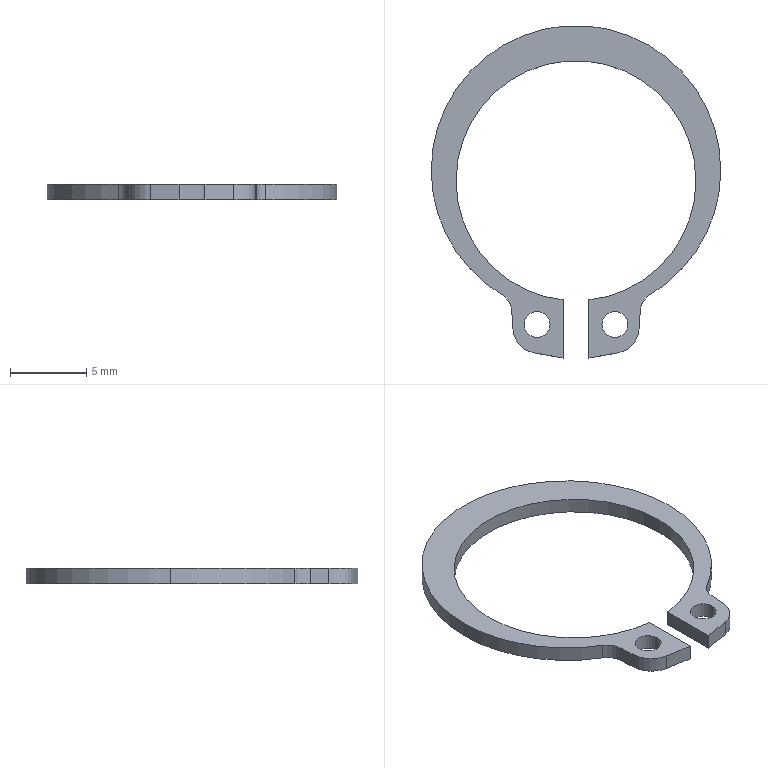Part | SolidWorks | features Extrusion 1, Fillet 1 | 1 solid | 22 faces | box 18.95 x 21.754 x 1 mm | volume 100.896 mm3 | cylinder 14 | plane 8 | commonest cylinder face diameters 1.7 x4 15.7 x3 18.95 x3 2.533 x2 3.4 x2
STEP:
#1=CARTESIAN_POINT('',(-3.4,-9.411,0.5));
#2=VERTEX_POINT('',#1);
#3=CARTESIAN_POINT('',(-1.7,-9.411,0.5));
#4=VERTEX_POINT('',#3);
#5=CARTESIAN_POINT('',(-2.55,-9.411,0.5));
#6=DIRECTION('',(0.,0.,1.));
#7=DIRECTION('',(-1.,0.,0.));
#8=AXIS2_PLACEMENT_3D('',#5,#6,#7);
#9=CIRCLE('',#8,0.85);
#10=EDGE_CURVE('',#2,#4,#9,.T.);
#11=ORIENTED_EDGE('',*,*,#10,.T.);
#12=CARTESIAN_POINT('',(-1.7,-9.411,-0.5));
#13=VERTEX_POINT('',#12);
#14=CARTESIAN_POINT('',(-1.7,-9.411,0.5));
#15=DIRECTION('',(0.,0.,-1.));
#16=VECTOR('',#15,1000.);
#17=LINE('',#14,#16);
#18=EDGE_CURVE('',#4,#13,#17,.T.);
#19=ORIENTED_EDGE('',*,*,#18,.T.);
#20=CARTESIAN_POINT('',(-3.4,-9.411,-0.5));
#21=VERTEX_POINT('',#20);
#22=CARTESIAN_POINT('',(-2.55,-9.411,-0.5));
#23=DIRECTION('',(0.,0.,1.));
#24=DIRECTION('',(-1.,0.,0.));
#25=AXIS2_PLACEMENT_3D('',#22,#23,#24);
#26=CIRCLE('',#25,0.85);
#27=EDGE_CURVE('',#21,#13,#26,.T.);
#28=ORIENTED_EDGE('',*,*,#27,.F.);
#29=CARTESIAN_POINT('',(-3.4,-9.411,0.5));
#30=DIRECTION('',(0.,0.,-1.));
#31=VECTOR('',#30,1000.);
#32=LINE('',#29,#31);
#33=EDGE_CURVE('',#2,#21,#32,.T.);
#34=ORIENTED_EDGE('',*,*,#33,.F.);
#35=EDGE_LOOP('',(#11,#19,#28,#34));
#36=FACE_OUTER_BOUND('',#35,.T.);
#37=CARTESIAN_POINT('',(-2.55,-9.411,0.5));
#38=DIRECTION('',(0.,0.,-1.));
#39=DIRECTION('',(-1.,0.,0.));
#40=AXIS2_PLACEMENT_3D('',#37,#38,#39);
#41=CYLINDRICAL_SURFACE('',#40,0.85);
#42=ADVANCED_FACE('',(#36),#41,.F.);
#43=CARTESIAN_POINT('',(1.7,-9.411,0.5));
#44=VERTEX_POINT('',#43);
#45=CARTESIAN_POINT('',(3.4,-9.411,0.5));
#46=VERTEX_POINT('',#45);
#47=CARTESIAN_POINT('',(2.55,-9.411,0.5));
#48=DIRECTION('',(0.,0.,1.));
#49=DIRECTION('',(1.,0.,0.));
#50=AXIS2_PLACEMENT_3D('',#47,#48,#49);
#51=CIRCLE('',#50,0.85);
#52=EDGE_CURVE('',#44,#46,#51,.T.);
#53=ORIENTED_EDGE('',*,*,#52,.T.);
#54=CARTESIAN_POINT('',(3.4,-9.411,-0.5));
#55=VERTEX_POINT('',#54);
#56=CARTESIAN_POINT('',(3.4,-9.411,0.5));
#57=DIRECTION('',(0.,0.,-1.));
#58=VECTOR('',#57,1000.);
#59=LINE('',#56,#58);
#60=EDGE_CURVE('',#46,#55,#59,.T.);
#61=ORIENTED_EDGE('',*,*,#60,.T.);
#62=CARTESIAN_POINT('',(1.7,-9.411,-0.5));
#63=VERTEX_POINT('',#62);
#64=CARTESIAN_POINT('',(2.55,-9.411,-0.5));
#65=DIRECTION('',(0.,0.,1.));
#66=DIRECTION('',(1.,0.,0.));
#67=AXIS2_PLACEMENT_3D('',#64,#65,#66);
#68=CIRCLE('',#67,0.85);
#69=EDGE_CURVE('',#63,#55,#68,.T.);
#70=ORIENTED_EDGE('',*,*,#69,.F.);
#71=CARTESIAN_POINT('',(1.7,-9.411,0.5));
#72=DIRECTION('',(0.,0.,-1.));
#73=VECTOR('',#72,1000.);
#74=LINE('',#71,#73);
#75=EDGE_CURVE('',#44,#63,#74,.T.);
#76=ORIENTED_EDGE('',*,*,#75,.F.);
#77=EDGE_LOOP('',(#53,#61,#70,#76));
#78=FACE_OUTER_BOUND('',#77,.T.);
#79=CARTESIAN_POINT('',(2.55,-9.411,0.5));
#80=DIRECTION('',(0.,0.,-1.));
#81=DIRECTION('',(-1.,0.,0.));
#82=AXIS2_PLACEMENT_3D('',#79,#80,#81);
#83=CYLINDRICAL_SURFACE('',#82,0.85);
#84=ADVANCED_FACE('',(#78),#83,.F.);
#85=CARTESIAN_POINT('',(7.85,0.,0.5));
#86=VERTEX_POINT('',#85);
#87=CARTESIAN_POINT('',(0.85,-7.804,0.5));
#88=VERTEX_POINT('',#87);
#89=CARTESIAN_POINT('',(0.,0.,0.5));
#90=DIRECTION('',(0.,0.,-1.));
#91=DIRECTION('',(1.,0.,0.));
#92=AXIS2_PLACEMENT_3D('',#89,#90,#91);
#93=CIRCLE('',#92,7.85);
#94=EDGE_CURVE('',#86,#88,#93,.T.);
#95=ORIENTED_EDGE('',*,*,#94,.F.);
#96=CARTESIAN_POINT('',(7.85,0.,-0.5));
#97=VERTEX_POINT('',#96);
#98=CARTESIAN_POINT('',(7.85,0.,0.5));
#99=DIRECTION('',(0.,0.,-1.));
#100=VECTOR('',#99,1000.);
#101=LINE('',#98,#100);
#102=EDGE_CURVE('',#86,#97,#101,.T.);
#103=ORIENTED_EDGE('',*,*,#102,.T.);
#104=CARTESIAN_POINT('',(0.85,-7.804,-0.5));
#105=VERTEX_POINT('',#104);
#106=CARTESIAN_POINT('',(0.,0.,-0.5));
#107=DIRECTION('',(0.,0.,-1.));
#108=DIRECTION('',(1.,0.,0.));
#109=AXIS2_PLACEMENT_3D('',#106,#107,#108);
#110=CIRCLE('',#109,7.85);
#111=EDGE_CURVE('',#97,#105,#110,.T.);
#112=ORIENTED_EDGE('',*,*,#111,.T.);
#113=CARTESIAN_POINT('',(0.85,-7.804,0.5));
#114=DIRECTION('',(0.,0.,-1.));
#115=VECTOR('',#114,1000.);
#116=LINE('',#113,#115);
#117=EDGE_CURVE('',#88,#105,#116,.T.);
#118=ORIENTED_EDGE('',*,*,#117,.F.);
#119=EDGE_LOOP('',(#95,#103,#112,#118));
#120=FACE_OUTER_BOUND('',#119,.T.);
#121=CARTESIAN_POINT('',(0.,0.,0.5));
#122=DIRECTION('',(0.,0.,-1.));
#123=DIRECTION('',(-1.,0.,0.));
#124=AXIS2_PLACEMENT_3D('',#121,#122,#123);
#125=CYLINDRICAL_SURFACE('',#124,7.85);
#126=ADVANCED_FACE('',(#120),#125,.F.);
#127=ORIENTED_EDGE('',*,*,#102,.F.);
#128=CARTESIAN_POINT('',(-7.85,0.,0.5));
#129=VERTEX_POINT('',#128);
#130=CARTESIAN_POINT('',(0.,0.,0.5));
#131=DIRECTION('',(0.,0.,-1.));
#132=DIRECTION('',(1.,0.,0.));
#133=AXIS2_PLACEMENT_3D('',#130,#131,#132);
#134=CIRCLE('',#133,7.85);
#135=EDGE_CURVE('',#129,#86,#134,.T.);
#136=ORIENTED_EDGE('',*,*,#135,.F.);
#137=CARTESIAN_POINT('',(-7.85,0.,-0.5));
#138=VERTEX_POINT('',#137);
#139=CARTESIAN_POINT('',(-7.85,0.,0.5));
#140=DIRECTION('',(0.,0.,-1.));
#141=VECTOR('',#140,1000.);
#142=LINE('',#139,#141);
#143=EDGE_CURVE('',#129,#138,#142,.T.);
#144=ORIENTED_EDGE('',*,*,#143,.T.);
#145=CARTESIAN_POINT('',(0.,0.,-0.5));
#146=DIRECTION('',(0.,0.,-1.));
#147=DIRECTION('',(1.,0.,0.));
#148=AXIS2_PLACEMENT_3D('',#145,#146,#147);
#149=CIRCLE('',#148,7.85);
#150=EDGE_CURVE('',#138,#97,#149,.T.);
#151=ORIENTED_EDGE('',*,*,#150,.T.);
#152=EDGE_LOOP('',(#127,#136,#144,#151));
#153=FACE_OUTER_BOUND('',#152,.T.);
#154=CARTESIAN_POINT('',(0.,0.,0.5));
#155=DIRECTION('',(0.,0.,-1.));
#156=DIRECTION('',(-1.,0.,0.));
#157=AXIS2_PLACEMENT_3D('',#154,#155,#156);
#158=CYLINDRICAL_SURFACE('',#157,7.85);
#159=ADVANCED_FACE('',(#153),#158,.F.);
#160=CARTESIAN_POINT('',(9.475,0.675,0.5));
#161=VERTEX_POINT('',#160);
#162=CARTESIAN_POINT('',(-9.475,0.675,0.5));
#163=VERTEX_POINT('',#162);
#164=CARTESIAN_POINT('',(0.,0.675,0.5));
#165=DIRECTION('',(0.,0.,1.));
#166=DIRECTION('',(1.,0.,0.));
#167=AXIS2_PLACEMENT_3D('',#164,#165,#166);
#168=CIRCLE('',#167,9.475);
#169=EDGE_CURVE('',#161,#163,#168,.T.);
#170=ORIENTED_EDGE('',*,*,#169,.F.);
#171=CARTESIAN_POINT('',(9.475,0.675,-0.5));
#172=VERTEX_POINT('',#171);
#173=CARTESIAN_POINT('',(9.475,0.675,0.5));
#174=DIRECTION('',(0.,0.,-1.));
#175=VECTOR('',#174,1000.);
#176=LINE('',#173,#175);
#177=EDGE_CURVE('',#161,#172,#176,.T.);
#178=ORIENTED_EDGE('',*,*,#177,.T.);
#179=CARTESIAN_POINT('',(-9.475,0.675,-0.5));
#180=VERTEX_POINT('',#179);
#181=CARTESIAN_POINT('',(0.,0.675,-0.5));
#182=DIRECTION('',(0.,0.,1.));
#183=DIRECTION('',(1.,0.,0.));
#184=AXIS2_PLACEMENT_3D('',#181,#182,#183);
#185=CIRCLE('',#184,9.475);
#186=EDGE_CURVE('',#172,#180,#185,.T.);
#187=ORIENTED_EDGE('',*,*,#186,.T.);
#188=CARTESIAN_POINT('',(-9.475,0.675,0.5));
#189=DIRECTION('',(0.,0.,-1.));
#190=VECTOR('',#189,1000.);
#191=LINE('',#188,#190);
#192=EDGE_CURVE('',#163,#180,#191,.T.);
#193=ORIENTED_EDGE('',*,*,#192,.F.);
#194=EDGE_LOOP('',(#170,#178,#187,#193));
#195=FACE_OUTER_BOUND('',#194,.T.);
#196=CARTESIAN_POINT('',(0.,0.675,0.5));
#197=DIRECTION('',(0.,0.,-1.));
#198=DIRECTION('',(-1.,0.,0.));
#199=AXIS2_PLACEMENT_3D('',#196,#197,#198);
#200=CYLINDRICAL_SURFACE('',#199,9.475);
#201=ADVANCED_FACE('',(#195),#200,.T.);
#202=CARTESIAN_POINT('',(-4.827,-7.479,0.5));
#203=VERTEX_POINT('',#202);
#204=CARTESIAN_POINT('',(0.,0.675,0.5));
#205=DIRECTION('',(0.,0.,1.));
#206=DIRECTION('',(1.,0.,0.));
#207=AXIS2_PLACEMENT_3D('',#204,#205,#206);
#208=CIRCLE('',#207,9.475);
#209=EDGE_CURVE('',#163,#203,#208,.T.);
#210=ORIENTED_EDGE('',*,*,#209,.F.);
#211=ORIENTED_EDGE('',*,*,#192,.T.);
#212=CARTESIAN_POINT('',(-4.827,-7.479,-0.5));
#213=VERTEX_POINT('',#212);
#214=CARTESIAN_POINT('',(0.,0.675,-0.5));
#215=DIRECTION('',(0.,0.,1.));
#216=DIRECTION('',(1.,0.,0.));
#217=AXIS2_PLACEMENT_3D('',#214,#215,#216);
#218=CIRCLE('',#217,9.475);
#219=EDGE_CURVE('',#180,#213,#218,.T.);
#220=ORIENTED_EDGE('',*,*,#219,.T.);
#221=CARTESIAN_POINT('',(-4.827,-7.479,0.5));
#222=DIRECTION('',(0.,0.,1.));
#223=VECTOR('',#222,1000.);
#224=LINE('',#221,#223);
#225=EDGE_CURVE('',#213,#203,#224,.T.);
#226=ORIENTED_EDGE('',*,*,#225,.T.);
#227=EDGE_LOOP('',(#210,#211,#220,#226));
#228=FACE_OUTER_BOUND('',#227,.T.);
#229=CARTESIAN_POINT('',(0.,0.675,0.5));
#230=DIRECTION('',(0.,0.,-1.));
#231=DIRECTION('',(-1.,0.,0.));
#232=AXIS2_PLACEMENT_3D('',#229,#230,#231);
#233=CYLINDRICAL_SURFACE('',#232,9.475);
#234=ADVANCED_FACE('',(#228),#233,.T.);
#235=ORIENTED_EDGE('',*,*,#52,.F.);
#236=CARTESIAN_POINT('',(2.55,-9.411,0.5));
#237=DIRECTION('',(0.,0.,1.));
#238=DIRECTION('',(1.,0.,0.));
#239=AXIS2_PLACEMENT_3D('',#236,#237,#238);
#240=CIRCLE('',#239,0.85);
#241=EDGE_CURVE('',#46,#44,#240,.T.);
#242=ORIENTED_EDGE('',*,*,#241,.F.);
#243=EDGE_LOOP('',(#235,#242));
#244=FACE_BOUND('',#243,.T.);
#245=CARTESIAN_POINT('',(2.732,-11.272,0.5));
#246=VERTEX_POINT('',#245);
#247=CARTESIAN_POINT('',(4.134,-9.701,0.5));
#248=VERTEX_POINT('',#247);
#249=CARTESIAN_POINT('',(2.437,-9.598,0.5));
#250=DIRECTION('',(0.,0.,1.));
#251=DIRECTION('',(1.,0.,0.));
#252=AXIS2_PLACEMENT_3D('',#249,#250,#251);
#253=CIRCLE('',#252,1.7);
#254=EDGE_CURVE('',#246,#248,#253,.T.);
#255=ORIENTED_EDGE('',*,*,#254,.T.);
#256=CARTESIAN_POINT('',(4.207,-8.492,0.5));
#257=VERTEX_POINT('',#256);
#258=CARTESIAN_POINT('',(4.134,-9.701,0.5));
#259=DIRECTION('',(0.06076,0.9982,0.));
#260=VECTOR('',#259,1000.);
#261=LINE('',#258,#260);
#262=EDGE_CURVE('',#248,#257,#261,.T.);
#263=ORIENTED_EDGE('',*,*,#262,.T.);
#264=CARTESIAN_POINT('',(4.827,-7.479,0.5));
#265=VERTEX_POINT('',#264);
#266=CARTESIAN_POINT('',(5.472,-8.569,0.5));
#267=DIRECTION('',(0.,0.,-1.));
#268=DIRECTION('',(1.,0.,0.));
#269=AXIS2_PLACEMENT_3D('',#266,#267,#268);
#270=CIRCLE('',#269,1.267);
#271=EDGE_CURVE('',#257,#265,#270,.T.);
#272=ORIENTED_EDGE('',*,*,#271,.T.);
#273=CARTESIAN_POINT('',(0.,0.675,0.5));
#274=DIRECTION('',(0.,0.,1.));
#275=DIRECTION('',(1.,0.,0.));
#276=AXIS2_PLACEMENT_3D('',#273,#274,#275);
#277=CIRCLE('',#276,9.475);
#278=EDGE_CURVE('',#265,#161,#277,.T.);
#279=ORIENTED_EDGE('',*,*,#278,.T.);
#280=ORIENTED_EDGE('',*,*,#169,.T.);
#281=ORIENTED_EDGE('',*,*,#209,.T.);
#282=CARTESIAN_POINT('',(-4.207,-8.492,0.5));
#283=VERTEX_POINT('',#282);
#284=CARTESIAN_POINT('',(-5.472,-8.569,0.5));
#285=DIRECTION('',(0.,0.,-1.));
#286=DIRECTION('',(1.,0.,0.));
#287=AXIS2_PLACEMENT_3D('',#284,#285,#286);
#288=CIRCLE('',#287,1.267);
#289=EDGE_CURVE('',#203,#283,#288,.T.);
#290=ORIENTED_EDGE('',*,*,#289,.T.);
#291=CARTESIAN_POINT('',(-4.134,-9.701,0.5));
#292=VERTEX_POINT('',#291);
#293=CARTESIAN_POINT('',(-4.134,-9.701,0.5));
#294=DIRECTION('',(0.06076,-0.9982,0.));
#295=VECTOR('',#294,1000.);
#296=LINE('',#293,#295);
#297=EDGE_CURVE('',#283,#292,#296,.T.);
#298=ORIENTED_EDGE('',*,*,#297,.T.);
#299=CARTESIAN_POINT('',(-2.732,-11.272,0.5));
#300=VERTEX_POINT('',#299);
#301=CARTESIAN_POINT('',(-2.437,-9.598,0.5));
#302=DIRECTION('',(0.,0.,1.));
#303=DIRECTION('',(-1.,0.,0.));
#304=AXIS2_PLACEMENT_3D('',#301,#302,#303);
#305=CIRCLE('',#304,1.7);
#306=EDGE_CURVE('',#292,#300,#305,.T.);
#307=ORIENTED_EDGE('',*,*,#306,.T.);
#308=CARTESIAN_POINT('',(-0.85,-11.604,0.5));
#309=VERTEX_POINT('',#308);
#310=CARTESIAN_POINT('',(-0.85,-11.604,0.5));
#311=DIRECTION('',(0.9848,-0.1736,0.));
#312=VECTOR('',#311,1000.);
#313=LINE('',#310,#312);
#314=EDGE_CURVE('',#300,#309,#313,.T.);
#315=ORIENTED_EDGE('',*,*,#314,.T.);
#316=CARTESIAN_POINT('',(-0.85,-7.804,0.5));
#317=VERTEX_POINT('',#316);
#318=CARTESIAN_POINT('',(-0.85,-7.804,0.5));
#319=DIRECTION('',(0.,1.,0.));
#320=VECTOR('',#319,1000.);
#321=LINE('',#318,#320);
#322=EDGE_CURVE('',#309,#317,#321,.T.);
#323=ORIENTED_EDGE('',*,*,#322,.T.);
#324=CARTESIAN_POINT('',(0.,0.,0.5));
#325=DIRECTION('',(0.,0.,-1.));
#326=DIRECTION('',(1.,0.,0.));
#327=AXIS2_PLACEMENT_3D('',#324,#325,#326);
#328=CIRCLE('',#327,7.85);
#329=EDGE_CURVE('',#317,#129,#328,.T.);
#330=ORIENTED_EDGE('',*,*,#329,.T.);
#331=ORIENTED_EDGE('',*,*,#135,.T.);
#332=ORIENTED_EDGE('',*,*,#94,.T.);
#333=CARTESIAN_POINT('',(0.85,-11.604,0.5));
#334=VERTEX_POINT('',#333);
#335=CARTESIAN_POINT('',(0.85,-7.804,0.5));
#336=DIRECTION('',(0.,-1.,0.));
#337=VECTOR('',#336,1000.);
#338=LINE('',#335,#337);
#339=EDGE_CURVE('',#88,#334,#338,.T.);
#340=ORIENTED_EDGE('',*,*,#339,.T.);
#341=CARTESIAN_POINT('',(0.85,-11.604,0.5));
#342=DIRECTION('',(0.9848,0.1736,0.));
#343=VECTOR('',#342,1000.);
#344=LINE('',#341,#343);
#345=EDGE_CURVE('',#334,#246,#344,.T.);
#346=ORIENTED_EDGE('',*,*,#345,.T.);
#347=EDGE_LOOP('',(#255,#263,#272,#279,#280,#281,#290,#298,#307,#315,#323,#330,#331,#332,#340,#346));
#348=FACE_OUTER_BOUND('',#347,.T.);
#349=ORIENTED_EDGE('',*,*,#10,.F.);
#350=CARTESIAN_POINT('',(-2.55,-9.411,0.5));
#351=DIRECTION('',(0.,0.,1.));
#352=DIRECTION('',(-1.,0.,0.));
#353=AXIS2_PLACEMENT_3D('',#350,#351,#352);
#354=CIRCLE('',#353,0.85);
#355=EDGE_CURVE('',#4,#2,#354,.T.);
#356=ORIENTED_EDGE('',*,*,#355,.F.);
#357=EDGE_LOOP('',(#349,#356));
#358=FACE_BOUND('',#357,.T.);
#359=CARTESIAN_POINT('',(2.437,-9.598,0.5));
#360=DIRECTION('',(0.,0.,1.));
#361=DIRECTION('',(1.,0.,0.));
#362=AXIS2_PLACEMENT_3D('',#359,#360,#361);
#363=PLANE('',#362);
#364=ADVANCED_FACE('',(#244,#348,#358),#363,.T.);
#365=CARTESIAN_POINT('',(2.732,-11.272,-0.5));
#366=VERTEX_POINT('',#365);
#367=CARTESIAN_POINT('',(4.134,-9.701,-0.5));
#368=VERTEX_POINT('',#367);
#369=CARTESIAN_POINT('',(2.437,-9.598,-0.5));
#370=DIRECTION('',(0.,0.,1.));
#371=DIRECTION('',(1.,0.,0.));
#372=AXIS2_PLACEMENT_3D('',#369,#370,#371);
#373=CIRCLE('',#372,1.7);
#374=EDGE_CURVE('',#366,#368,#373,.T.);
#375=ORIENTED_EDGE('',*,*,#374,.F.);
#376=CARTESIAN_POINT('',(0.85,-11.604,-0.5));
#377=VERTEX_POINT('',#376);
#378=CARTESIAN_POINT('',(0.85,-11.604,-0.5));
#379=DIRECTION('',(0.9848,0.1736,0.));
#380=VECTOR('',#379,1000.);
#381=LINE('',#378,#380);
#382=EDGE_CURVE('',#377,#366,#381,.T.);
#383=ORIENTED_EDGE('',*,*,#382,.F.);
#384=CARTESIAN_POINT('',(0.85,-7.804,-0.5));
#385=DIRECTION('',(0.,-1.,0.));
#386=VECTOR('',#385,1000.);
#387=LINE('',#384,#386);
#388=EDGE_CURVE('',#105,#377,#387,.T.);
#389=ORIENTED_EDGE('',*,*,#388,.F.);
#390=ORIENTED_EDGE('',*,*,#111,.F.);
#391=ORIENTED_EDGE('',*,*,#150,.F.);
#392=CARTESIAN_POINT('',(-0.85,-7.804,-0.5));
#393=VERTEX_POINT('',#392);
#394=CARTESIAN_POINT('',(0.,0.,-0.5));
#395=DIRECTION('',(0.,0.,-1.));
#396=DIRECTION('',(1.,0.,0.));
#397=AXIS2_PLACEMENT_3D('',#394,#395,#396);
#398=CIRCLE('',#397,7.85);
#399=EDGE_CURVE('',#393,#138,#398,.T.);
#400=ORIENTED_EDGE('',*,*,#399,.F.);
#401=CARTESIAN_POINT('',(-0.85,-11.604,-0.5));
#402=VERTEX_POINT('',#401);
#403=CARTESIAN_POINT('',(-0.85,-7.804,-0.5));
#404=DIRECTION('',(0.,1.,0.));
#405=VECTOR('',#404,1000.);
#406=LINE('',#403,#405);
#407=EDGE_CURVE('',#402,#393,#406,.T.);
#408=ORIENTED_EDGE('',*,*,#407,.F.);
#409=CARTESIAN_POINT('',(-2.732,-11.272,-0.5));
#410=VERTEX_POINT('',#409);
#411=CARTESIAN_POINT('',(-0.85,-11.604,-0.5));
#412=DIRECTION('',(0.9848,-0.1736,0.));
#413=VECTOR('',#412,1000.);
#414=LINE('',#411,#413);
#415=EDGE_CURVE('',#410,#402,#414,.T.);
#416=ORIENTED_EDGE('',*,*,#415,.F.);
#417=CARTESIAN_POINT('',(-4.134,-9.701,-0.5));
#418=VERTEX_POINT('',#417);
#419=CARTESIAN_POINT('',(-2.437,-9.598,-0.5));
#420=DIRECTION('',(0.,0.,1.));
#421=DIRECTION('',(-1.,0.,0.));
#422=AXIS2_PLACEMENT_3D('',#419,#420,#421);
#423=CIRCLE('',#422,1.7);
#424=EDGE_CURVE('',#418,#410,#423,.T.);
#425=ORIENTED_EDGE('',*,*,#424,.F.);
#426=CARTESIAN_POINT('',(-4.207,-8.492,-0.5));
#427=VERTEX_POINT('',#426);
#428=CARTESIAN_POINT('',(-4.134,-9.701,-0.5));
#429=DIRECTION('',(0.06076,-0.9982,0.));
#430=VECTOR('',#429,1000.);
#431=LINE('',#428,#430);
#432=EDGE_CURVE('',#427,#418,#431,.T.);
#433=ORIENTED_EDGE('',*,*,#432,.F.);
#434=CARTESIAN_POINT('',(-5.472,-8.569,-0.5));
#435=DIRECTION('',(0.,0.,1.));
#436=DIRECTION('',(1.,0.,0.));
#437=AXIS2_PLACEMENT_3D('',#434,#435,#436);
#438=CIRCLE('',#437,1.267);
#439=EDGE_CURVE('',#427,#213,#438,.T.);
#440=ORIENTED_EDGE('',*,*,#439,.T.);
#441=ORIENTED_EDGE('',*,*,#219,.F.);
#442=ORIENTED_EDGE('',*,*,#186,.F.);
#443=CARTESIAN_POINT('',(4.827,-7.479,-0.5));
#444=VERTEX_POINT('',#443);
#445=CARTESIAN_POINT('',(0.,0.675,-0.5));
#446=DIRECTION('',(0.,0.,1.));
#447=DIRECTION('',(1.,0.,0.));
#448=AXIS2_PLACEMENT_3D('',#445,#446,#447);
#449=CIRCLE('',#448,9.475);
#450=EDGE_CURVE('',#444,#172,#449,.T.);
#451=ORIENTED_EDGE('',*,*,#450,.F.);
#452=CARTESIAN_POINT('',(4.207,-8.492,-0.5));
#453=VERTEX_POINT('',#452);
#454=CARTESIAN_POINT('',(5.472,-8.569,-0.5));
#455=DIRECTION('',(0.,0.,1.));
#456=DIRECTION('',(1.,0.,0.));
#457=AXIS2_PLACEMENT_3D('',#454,#455,#456);
#458=CIRCLE('',#457,1.267);
#459=EDGE_CURVE('',#444,#453,#458,.T.);
#460=ORIENTED_EDGE('',*,*,#459,.T.);
#461=CARTESIAN_POINT('',(4.134,-9.701,-0.5));
#462=DIRECTION('',(0.06076,0.9982,0.));
#463=VECTOR('',#462,1000.);
#464=LINE('',#461,#463);
#465=EDGE_CURVE('',#368,#453,#464,.T.);
#466=ORIENTED_EDGE('',*,*,#465,.F.);
#467=EDGE_LOOP('',(#375,#383,#389,#390,#391,#400,#408,#416,#425,#433,#440,#441,#442,#451,#460,#466));
#468=FACE_OUTER_BOUND('',#467,.T.);
#469=ORIENTED_EDGE('',*,*,#69,.T.);
#470=CARTESIAN_POINT('',(2.55,-9.411,-0.5));
#471=DIRECTION('',(0.,0.,1.));
#472=DIRECTION('',(1.,0.,0.));
#473=AXIS2_PLACEMENT_3D('',#470,#471,#472);
#474=CIRCLE('',#473,0.85);
#475=EDGE_CURVE('',#55,#63,#474,.T.);
#476=ORIENTED_EDGE('',*,*,#475,.T.);
#477=EDGE_LOOP('',(#469,#476));
#478=FACE_BOUND('',#477,.T.);
#479=ORIENTED_EDGE('',*,*,#27,.T.);
#480=CARTESIAN_POINT('',(-2.55,-9.411,-0.5));
#481=DIRECTION('',(0.,0.,1.));
#482=DIRECTION('',(-1.,0.,0.));
#483=AXIS2_PLACEMENT_3D('',#480,#481,#482);
#484=CIRCLE('',#483,0.85);
#485=EDGE_CURVE('',#13,#21,#484,.T.);
#486=ORIENTED_EDGE('',*,*,#485,.T.);
#487=EDGE_LOOP('',(#479,#486));
#488=FACE_BOUND('',#487,.T.);
#489=CARTESIAN_POINT('',(2.437,-9.598,-0.5));
#490=DIRECTION('',(0.,0.,1.));
#491=DIRECTION('',(1.,0.,0.));
#492=AXIS2_PLACEMENT_3D('',#489,#490,#491);
#493=PLANE('',#492);
#494=ADVANCED_FACE('',(#468,#478,#488),#493,.F.);
#495=ORIENTED_EDGE('',*,*,#374,.T.);
#496=CARTESIAN_POINT('',(4.134,-9.701,0.5));
#497=DIRECTION('',(0.,0.,-1.));
#498=VECTOR('',#497,1000.);
#499=LINE('',#496,#498);
#500=EDGE_CURVE('',#248,#368,#499,.T.);
#501=ORIENTED_EDGE('',*,*,#500,.F.);
#502=ORIENTED_EDGE('',*,*,#254,.F.);
#503=CARTESIAN_POINT('',(2.732,-11.272,0.5));
#504=DIRECTION('',(0.,0.,-1.));
#505=VECTOR('',#504,1000.);
#506=LINE('',#503,#505);
#507=EDGE_CURVE('',#246,#366,#506,.T.);
#508=ORIENTED_EDGE('',*,*,#507,.T.);
#509=EDGE_LOOP('',(#495,#501,#502,#508));
#510=FACE_OUTER_BOUND('',#509,.T.);
#511=CARTESIAN_POINT('',(2.437,-9.598,0.5));
#512=DIRECTION('',(0.,0.,-1.));
#513=DIRECTION('',(-1.,0.,0.));
#514=AXIS2_PLACEMENT_3D('',#511,#512,#513);
#515=CYLINDRICAL_SURFACE('',#514,1.7);
#516=ADVANCED_FACE('',(#510),#515,.T.);
#517=ORIENTED_EDGE('',*,*,#465,.T.);
#518=CARTESIAN_POINT('',(4.207,-8.492,0.5));
#519=DIRECTION('',(0.,0.,1.));
#520=VECTOR('',#519,1000.);
#521=LINE('',#518,#520);
#522=EDGE_CURVE('',#453,#257,#521,.T.);
#523=ORIENTED_EDGE('',*,*,#522,.T.);
#524=ORIENTED_EDGE('',*,*,#262,.F.);
#525=ORIENTED_EDGE('',*,*,#500,.T.);
#526=EDGE_LOOP('',(#517,#523,#524,#525));
#527=FACE_OUTER_BOUND('',#526,.T.);
#528=CARTESIAN_POINT('',(4.134,-9.701,0.5));
#529=DIRECTION('',(-0.9982,0.06076,0.));
#530=DIRECTION('',(-0.06076,-0.9982,0.));
#531=AXIS2_PLACEMENT_3D('',#528,#529,#530);
#532=PLANE('',#531);
#533=ADVANCED_FACE('',(#527),#532,.F.);
#534=ORIENTED_EDGE('',*,*,#177,.F.);
#535=ORIENTED_EDGE('',*,*,#278,.F.);
#536=CARTESIAN_POINT('',(4.827,-7.479,0.5));
#537=DIRECTION('',(0.,0.,-1.));
#538=VECTOR('',#537,1000.);
#539=LINE('',#536,#538);
#540=EDGE_CURVE('',#265,#444,#539,.T.);
#541=ORIENTED_EDGE('',*,*,#540,.T.);
#542=ORIENTED_EDGE('',*,*,#450,.T.);
#543=EDGE_LOOP('',(#534,#535,#541,#542));
#544=FACE_OUTER_BOUND('',#543,.T.);
#545=CARTESIAN_POINT('',(0.,0.675,0.5));
#546=DIRECTION('',(0.,0.,-1.));
#547=DIRECTION('',(-1.,0.,0.));
#548=AXIS2_PLACEMENT_3D('',#545,#546,#547);
#549=CYLINDRICAL_SURFACE('',#548,9.475);
#550=ADVANCED_FACE('',(#544),#549,.T.);
#551=ORIENTED_EDGE('',*,*,#297,.F.);
#552=CARTESIAN_POINT('',(-4.207,-8.492,-0.5));
#553=DIRECTION('',(0.,0.,-1.));
#554=VECTOR('',#553,1000.);
#555=LINE('',#552,#554);
#556=EDGE_CURVE('',#283,#427,#555,.T.);
#557=ORIENTED_EDGE('',*,*,#556,.T.);
#558=ORIENTED_EDGE('',*,*,#432,.T.);
#559=CARTESIAN_POINT('',(-4.134,-9.701,0.5));
#560=DIRECTION('',(0.,0.,-1.));
#561=VECTOR('',#560,1000.);
#562=LINE('',#559,#561);
#563=EDGE_CURVE('',#292,#418,#562,.T.);
#564=ORIENTED_EDGE('',*,*,#563,.F.);
#565=EDGE_LOOP('',(#551,#557,#558,#564));
#566=FACE_OUTER_BOUND('',#565,.T.);
#567=CARTESIAN_POINT('',(-4.134,-9.701,0.5));
#568=DIRECTION('',(0.9982,0.06076,0.));
#569=DIRECTION('',(-0.06076,0.9982,0.));
#570=AXIS2_PLACEMENT_3D('',#567,#568,#569);
#571=PLANE('',#570);
#572=ADVANCED_FACE('',(#566),#571,.F.);
#573=ORIENTED_EDGE('',*,*,#424,.T.);
#574=CARTESIAN_POINT('',(-2.732,-11.272,0.5));
#575=DIRECTION('',(0.,0.,-1.));
#576=VECTOR('',#575,1000.);
#577=LINE('',#574,#576);
#578=EDGE_CURVE('',#300,#410,#577,.T.);
#579=ORIENTED_EDGE('',*,*,#578,.F.);
#580=ORIENTED_EDGE('',*,*,#306,.F.);
#581=ORIENTED_EDGE('',*,*,#563,.T.);
#582=EDGE_LOOP('',(#573,#579,#580,#581));
#583=FACE_OUTER_BOUND('',#582,.T.);
#584=CARTESIAN_POINT('',(-2.437,-9.598,0.5));
#585=DIRECTION('',(0.,0.,-1.));
#586=DIRECTION('',(-1.,0.,0.));
#587=AXIS2_PLACEMENT_3D('',#584,#585,#586);
#588=CYLINDRICAL_SURFACE('',#587,1.7);
#589=ADVANCED_FACE('',(#583),#588,.T.);
#590=ORIENTED_EDGE('',*,*,#415,.T.);
#591=CARTESIAN_POINT('',(-0.85,-11.604,0.5));
#592=DIRECTION('',(0.,0.,-1.));
#593=VECTOR('',#592,1000.);
#594=LINE('',#591,#593);
#595=EDGE_CURVE('',#309,#402,#594,.T.);
#596=ORIENTED_EDGE('',*,*,#595,.F.);
#597=ORIENTED_EDGE('',*,*,#314,.F.);
#598=ORIENTED_EDGE('',*,*,#578,.T.);
#599=EDGE_LOOP('',(#590,#596,#597,#598));
#600=FACE_OUTER_BOUND('',#599,.T.);
#601=CARTESIAN_POINT('',(-0.85,-11.604,0.5));
#602=DIRECTION('',(0.1736,0.9848,0.));
#603=DIRECTION('',(-0.9848,0.1736,0.));
#604=AXIS2_PLACEMENT_3D('',#601,#602,#603);
#605=PLANE('',#604);
#606=ADVANCED_FACE('',(#600),#605,.F.);
#607=ORIENTED_EDGE('',*,*,#407,.T.);
#608=CARTESIAN_POINT('',(-0.85,-7.804,0.5));
#609=DIRECTION('',(0.,0.,-1.));
#610=VECTOR('',#609,1000.);
#611=LINE('',#608,#610);
#612=EDGE_CURVE('',#317,#393,#611,.T.);
#613=ORIENTED_EDGE('',*,*,#612,.F.);
#614=ORIENTED_EDGE('',*,*,#322,.F.);
#615=ORIENTED_EDGE('',*,*,#595,.T.);
#616=EDGE_LOOP('',(#607,#613,#614,#615));
#617=FACE_OUTER_BOUND('',#616,.T.);
#618=CARTESIAN_POINT('',(-0.85,-7.804,0.5));
#619=DIRECTION('',(-1.,0.,0.));
#620=DIRECTION('',(0.,-1.,0.));
#621=AXIS2_PLACEMENT_3D('',#618,#619,#620);
#622=PLANE('',#621);
#623=ADVANCED_FACE('',(#617),#622,.F.);
#624=ORIENTED_EDGE('',*,*,#143,.F.);
#625=ORIENTED_EDGE('',*,*,#329,.F.);
#626=ORIENTED_EDGE('',*,*,#612,.T.);
#627=ORIENTED_EDGE('',*,*,#399,.T.);
#628=EDGE_LOOP('',(#624,#625,#626,#627));
#629=FACE_OUTER_BOUND('',#628,.T.);
#630=CARTESIAN_POINT('',(0.,0.,0.5));
#631=DIRECTION('',(0.,0.,-1.));
#632=DIRECTION('',(-1.,0.,0.));
#633=AXIS2_PLACEMENT_3D('',#630,#631,#632);
#634=CYLINDRICAL_SURFACE('',#633,7.85);
#635=ADVANCED_FACE('',(#629),#634,.F.);
#636=ORIENTED_EDGE('',*,*,#388,.T.);
#637=CARTESIAN_POINT('',(0.85,-11.604,0.5));
#638=DIRECTION('',(0.,0.,-1.));
#639=VECTOR('',#638,1000.);
#640=LINE('',#637,#639);
#641=EDGE_CURVE('',#334,#377,#640,.T.);
#642=ORIENTED_EDGE('',*,*,#641,.F.);
#643=ORIENTED_EDGE('',*,*,#339,.F.);
#644=ORIENTED_EDGE('',*,*,#117,.T.);
#645=EDGE_LOOP('',(#636,#642,#643,#644));
#646=FACE_OUTER_BOUND('',#645,.T.);
#647=CARTESIAN_POINT('',(0.85,-7.804,0.5));
#648=DIRECTION('',(1.,0.,0.));
#649=DIRECTION('',(0.,0.,-1.));
#650=AXIS2_PLACEMENT_3D('',#647,#648,#649);
#651=PLANE('',#650);
#652=ADVANCED_FACE('',(#646),#651,.F.);
#653=ORIENTED_EDGE('',*,*,#382,.T.);
#654=ORIENTED_EDGE('',*,*,#507,.F.);
#655=ORIENTED_EDGE('',*,*,#345,.F.);
#656=ORIENTED_EDGE('',*,*,#641,.T.);
#657=EDGE_LOOP('',(#653,#654,#655,#656));
#658=FACE_OUTER_BOUND('',#657,.T.);
#659=CARTESIAN_POINT('',(0.85,-11.604,0.5));
#660=DIRECTION('',(-0.1736,0.9848,0.));
#661=DIRECTION('',(-0.9848,-0.1736,0.));
#662=AXIS2_PLACEMENT_3D('',#659,#660,#661);
#663=PLANE('',#662);
#664=ADVANCED_FACE('',(#658),#663,.F.);
#665=ORIENTED_EDGE('',*,*,#60,.F.);
#666=ORIENTED_EDGE('',*,*,#241,.T.);
#667=ORIENTED_EDGE('',*,*,#75,.T.);
#668=ORIENTED_EDGE('',*,*,#475,.F.);
#669=EDGE_LOOP('',(#665,#666,#667,#668));
#670=FACE_OUTER_BOUND('',#669,.T.);
#671=CARTESIAN_POINT('',(2.55,-9.411,0.5));
#672=DIRECTION('',(0.,0.,-1.));
#673=DIRECTION('',(-1.,0.,0.));
#674=AXIS2_PLACEMENT_3D('',#671,#672,#673);
#675=CYLINDRICAL_SURFACE('',#674,0.85);
#676=ADVANCED_FACE('',(#670),#675,.F.);
#677=ORIENTED_EDGE('',*,*,#18,.F.);
#678=ORIENTED_EDGE('',*,*,#355,.T.);
#679=ORIENTED_EDGE('',*,*,#33,.T.);
#680=ORIENTED_EDGE('',*,*,#485,.F.);
#681=EDGE_LOOP('',(#677,#678,#679,#680));
#682=FACE_OUTER_BOUND('',#681,.T.);
#683=CARTESIAN_POINT('',(-2.55,-9.411,0.5));
#684=DIRECTION('',(0.,0.,-1.));
#685=DIRECTION('',(-1.,0.,0.));
#686=AXIS2_PLACEMENT_3D('',#683,#684,#685);
#687=CYLINDRICAL_SURFACE('',#686,0.85);
#688=ADVANCED_FACE('',(#682),#687,.F.);
#689=ORIENTED_EDGE('',*,*,#289,.F.);
#690=ORIENTED_EDGE('',*,*,#225,.F.);
#691=ORIENTED_EDGE('',*,*,#439,.F.);
#692=ORIENTED_EDGE('',*,*,#556,.F.);
#693=EDGE_LOOP('',(#689,#690,#691,#692));
#694=FACE_OUTER_BOUND('',#693,.T.);
#695=CARTESIAN_POINT('',(-5.472,-8.569,0.5));
#696=DIRECTION('',(0.,0.,-1.));
#697=DIRECTION('',(-1.,0.,0.));
#698=AXIS2_PLACEMENT_3D('',#695,#696,#697);
#699=CYLINDRICAL_SURFACE('',#698,1.267);
#700=ADVANCED_FACE('',(#694),#699,.F.);
#701=ORIENTED_EDGE('',*,*,#271,.F.);
#702=ORIENTED_EDGE('',*,*,#522,.F.);
#703=ORIENTED_EDGE('',*,*,#459,.F.);
#704=ORIENTED_EDGE('',*,*,#540,.F.);
#705=EDGE_LOOP('',(#701,#702,#703,#704));
#706=FACE_OUTER_BOUND('',#705,.T.);
#707=CARTESIAN_POINT('',(5.472,-8.569,0.5));
#708=DIRECTION('',(0.,0.,-1.));
#709=DIRECTION('',(-1.,0.,0.));
#710=AXIS2_PLACEMENT_3D('',#707,#708,#709);
#711=CYLINDRICAL_SURFACE('',#710,1.267);
#712=ADVANCED_FACE('',(#706),#711,.F.);
#713=CLOSED_SHELL('',(#42,#84,#126,#159,#201,#234,#364,#494,#516,#533,#550,#572,#589,#606,#623,#635,#652,#664,#676,#688,#700,#712));
#714=MANIFOLD_SOLID_BREP('',#713);
#715=CARTESIAN_POINT('',(0.,0.,0.));
#716=DIRECTION('',(0.,0.,1.));
#717=DIRECTION('',(1.,0.,0.));
#718=AXIS2_PLACEMENT_3D('',#715,#716,#717);
#719=(LENGTH_UNIT()NAMED_UNIT(*)SI_UNIT(.MILLI.,.METRE.));
#720=UNCERTAINTY_MEASURE_WITH_UNIT(LENGTH_MEASURE(0.00001),#719,'','');
#721=(NAMED_UNIT(*)PLANE_ANGLE_UNIT()SI_UNIT($,.RADIAN.));
#722=(NAMED_UNIT(*)SI_UNIT($,.STERADIAN.)SOLID_ANGLE_UNIT());
#723=(GEOMETRIC_REPRESENTATION_CONTEXT(3)GLOBAL_UNCERTAINTY_ASSIGNED_CONTEXT((#720))GLOBAL_UNIT_ASSIGNED_CONTEXT((#719,#721,#722))REPRESENTATION_CONTEXT('',''));
#724=ADVANCED_BREP_SHAPE_REPRESENTATION('',(#714,#718),#723);